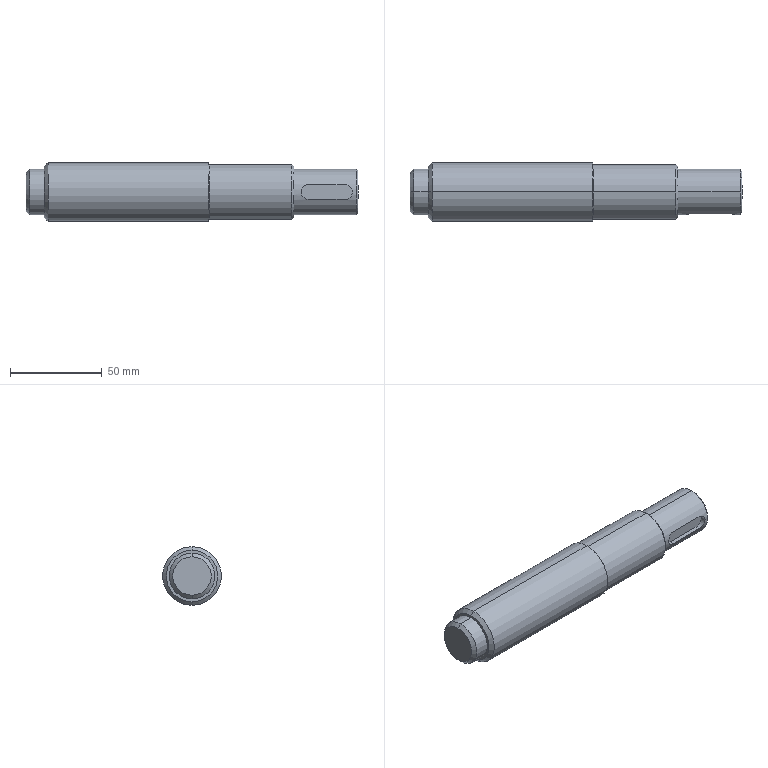Part | SolidWorks | features BaseBody 1 | 1 solid | 32 faces | box 181 x 32 x 32 mm | volume 124690 mm3 | cylinder 12 | cone 10 | plane 8 | spline 2 | commonest cylinder face diameters 25 x4 6.647 x2 8 x2 30 x2 32 x2
STEP:
#1=CARTESIAN_POINT('',(99.5,0.,15.5));
#2=VERTEX_POINT('',#1);
#3=CARTESIAN_POINT('',(99.5,0.,-15.5));
#4=VERTEX_POINT('',#3);
#5=CARTESIAN_POINT('',(99.5,0.,15.5));
#6=CARTESIAN_POINT('',(99.5,0.4739,15.5));
#7=CARTESIAN_POINT('',(99.5,1.182,15.468));
#8=CARTESIAN_POINT('',(99.5,2.003,15.373));
#9=CARTESIAN_POINT('',(99.5,2.412,15.312));
#10=CARTESIAN_POINT('',(99.5,2.616,15.278));
#11=CARTESIAN_POINT('',(99.5,2.704,15.262));
#12=CARTESIAN_POINT('',(99.5,2.762,15.252));
#13=CARTESIAN_POINT('',(99.5,2.79,15.247));
#14=CARTESIAN_POINT('',(99.5,3.315,15.15));
#15=CARTESIAN_POINT('',(99.5,4.046,14.978));
#16=CARTESIAN_POINT('',(99.5,4.881,14.715));
#17=CARTESIAN_POINT('',(99.5,5.295,14.569));
#18=CARTESIAN_POINT('',(99.5,5.501,14.491));
#19=CARTESIAN_POINT('',(99.5,5.588,14.458));
#20=CARTESIAN_POINT('',(99.5,5.647,14.435));
#21=CARTESIAN_POINT('',(99.5,5.675,14.424));
#22=CARTESIAN_POINT('',(99.5,6.192,14.219));
#23=CARTESIAN_POINT('',(99.5,6.905,13.895));
#24=CARTESIAN_POINT('',(99.5,7.704,13.455));
#25=CARTESIAN_POINT('',(99.5,8.095,13.219));
#26=CARTESIAN_POINT('',(99.5,8.262,13.115));
#27=CARTESIAN_POINT('',(99.5,8.372,13.045));
#28=CARTESIAN_POINT('',(99.5,8.426,13.01));
#29=CARTESIAN_POINT('',(99.5,9.377,12.388));
#30=CARTESIAN_POINT('',(99.5,10.204,11.717));
#31=CARTESIAN_POINT('',(99.5,11.338,10.582));
#32=CARTESIAN_POINT('',(99.5,11.874,9.989));
#33=CARTESIAN_POINT('',(99.5,12.442,9.25));
#34=CARTESIAN_POINT('',(99.5,12.712,8.87));
#35=CARTESIAN_POINT('',(99.5,12.825,8.704));
#36=CARTESIAN_POINT('',(99.5,12.9,8.593));
#37=CARTESIAN_POINT('',(99.5,12.938,8.537));
#38=CARTESIAN_POINT('',(99.5,13.26,8.043));
#39=CARTESIAN_POINT('',(99.5,13.655,7.368));
#40=CARTESIAN_POINT('',(99.5,14.054,6.547));
#41=CARTESIAN_POINT('',(99.5,14.238,6.129));
#42=CARTESIAN_POINT('',(99.5,14.326,5.918));
#43=CARTESIAN_POINT('',(99.5,14.363,5.827));
#44=CARTESIAN_POINT('',(99.5,14.388,5.766));
#45=CARTESIAN_POINT('',(99.5,14.4,5.735));
#46=CARTESIAN_POINT('',(99.5,14.597,5.238));
#47=CARTESIAN_POINT('',(99.5,14.839,4.527));
#48=CARTESIAN_POINT('',(99.5,15.061,3.68));
#49=CARTESIAN_POINT('',(99.5,15.156,3.252));
#50=CARTESIAN_POINT('',(99.5,15.2,3.036));
#51=CARTESIAN_POINT('',(99.5,15.218,2.944));
#52=CARTESIAN_POINT('',(99.5,15.23,2.882));
#53=CARTESIAN_POINT('',(99.5,15.236,2.85));
#54=CARTESIAN_POINT('',(99.5,15.414,1.888));
#55=CARTESIAN_POINT('',(99.5,15.5,0.9479));
#56=CARTESIAN_POINT('',(99.5,15.5,-0.4739));
#57=CARTESIAN_POINT('',(99.5,15.478,-0.9462));
#58=CARTESIAN_POINT('',(99.5,15.414,-1.651));
#59=CARTESIAN_POINT('',(99.5,15.373,-2.003));
#60=CARTESIAN_POINT('',(99.5,15.312,-2.412));
#61=CARTESIAN_POINT('',(99.5,15.278,-2.616));
#62=CARTESIAN_POINT('',(99.5,15.262,-2.704));
#63=CARTESIAN_POINT('',(99.5,15.252,-2.762));
#64=CARTESIAN_POINT('',(99.5,15.247,-2.79));
#65=CARTESIAN_POINT('',(99.5,15.15,-3.315));
#66=CARTESIAN_POINT('',(99.5,14.978,-4.046));
#67=CARTESIAN_POINT('',(99.5,14.715,-4.881));
#68=CARTESIAN_POINT('',(99.5,14.569,-5.295));
#69=CARTESIAN_POINT('',(99.5,14.491,-5.501));
#70=CARTESIAN_POINT('',(99.5,14.458,-5.588));
#71=CARTESIAN_POINT('',(99.5,14.435,-5.647));
#72=CARTESIAN_POINT('',(99.5,14.424,-5.675));
#73=CARTESIAN_POINT('',(99.5,14.219,-6.192));
#74=CARTESIAN_POINT('',(99.5,13.895,-6.905));
#75=CARTESIAN_POINT('',(99.5,13.455,-7.704));
#76=CARTESIAN_POINT('',(99.5,13.219,-8.095));
#77=CARTESIAN_POINT('',(99.5,13.115,-8.262));
#78=CARTESIAN_POINT('',(99.5,13.045,-8.372));
#79=CARTESIAN_POINT('',(99.5,13.01,-8.426));
#80=CARTESIAN_POINT('',(99.5,12.388,-9.377));
#81=CARTESIAN_POINT('',(99.5,11.717,-10.204));
#82=CARTESIAN_POINT('',(99.5,10.582,-11.338));
#83=CARTESIAN_POINT('',(99.5,9.989,-11.874));
#84=CARTESIAN_POINT('',(99.5,9.25,-12.442));
#85=CARTESIAN_POINT('',(99.5,8.87,-12.712));
#86=CARTESIAN_POINT('',(99.5,8.704,-12.825));
#87=CARTESIAN_POINT('',(99.5,8.593,-12.9));
#88=CARTESIAN_POINT('',(99.5,8.537,-12.938));
#89=CARTESIAN_POINT('',(99.5,8.043,-13.26));
#90=CARTESIAN_POINT('',(99.5,7.368,-13.655));
#91=CARTESIAN_POINT('',(99.5,6.547,-14.054));
#92=CARTESIAN_POINT('',(99.5,6.129,-14.238));
#93=CARTESIAN_POINT('',(99.5,5.918,-14.326));
#94=CARTESIAN_POINT('',(99.5,5.827,-14.363));
#95=CARTESIAN_POINT('',(99.5,5.766,-14.388));
#96=CARTESIAN_POINT('',(99.5,5.735,-14.4));
#97=CARTESIAN_POINT('',(99.5,5.238,-14.597));
#98=CARTESIAN_POINT('',(99.5,4.527,-14.839));
#99=CARTESIAN_POINT('',(99.5,3.68,-15.061));
#100=CARTESIAN_POINT('',(99.5,3.252,-15.156));
#101=CARTESIAN_POINT('',(99.5,3.036,-15.2));
#102=CARTESIAN_POINT('',(99.5,2.944,-15.218));
#103=CARTESIAN_POINT('',(99.5,2.882,-15.23));
#104=CARTESIAN_POINT('',(99.5,2.85,-15.236));
#105=CARTESIAN_POINT('',(99.5,1.889,-15.414));
#106=CARTESIAN_POINT('',(99.5,0.9477,-15.5));
#107=CARTESIAN_POINT('',(99.5,0.,-15.5));
#108=B_SPLINE_CURVE_WITH_KNOTS('',3,(#5,#6,#7,#8,#9,#10,#11,#12,#13,#14,#15,#16,#17,#18,#19,#20,#21,#22,#23,#24,#25,#26,#27,#28,#29,#30,#31,#32,#33,#34,#35,#36,#37,#38,#39,#40,#41,#42,#43,#44,#45,#46,#47,#48,#49,#50,#51,#52,#53,#54,#55,#56,#57,#58,#59,#60,#61,#62,#63,#64,#65,#66,#67,#68,#69,#70,#71,#72,#73,#74,#75,#76,#77,#78,#79,#80,#81,#82,#83,#84,#85,#86,#87,#88,#89,#90,#91,#92,#93,#94,#95,#96,#97,#98,#99,#100,#101,#102,#103,#104,#105,#106,#107),.UNSPECIFIED.,.F.,.F.,(4,1,1,1,1,2,2,1,1,1,1,2,2,1,1,1,2,2,2,1,1,1,2,2,1,1,1,1,2,2,1,1,1,1,2,2,2,2,1,1,1,2,2,1,1,1,1,2,2,1,1,1,2,2,2,1,1,1,2,2,1,1,1,1,2,2,1,1,1,1,2,2,4),(0.75,0.7656,0.7734,0.7773,0.7793,0.7803,0.7813,0.7969,0.8047,0.8086,0.8105,0.8115,0.8125,0.8281,0.8359,0.8398,0.8418,0.8438,0.875,0.8906,0.8984,0.9023,0.9043,0.9063,0.9219,0.9297,0.9336,0.9355,0.9365,0.9375,0.9531,0.9609,0.9648,0.9668,0.9678,0.9688,1.,1.016,1.023,1.027,1.029,1.03,1.031,1.047,1.055,1.059,1.061,1.062,1.063,1.078,1.086,1.09,1.092,1.094,1.125,1.141,1.148,1.152,1.154,1.156,1.172,1.18,1.184,1.186,1.187,1.188,1.203,1.211,1.215,1.217,1.218,1.219,1.25),.UNSPECIFIED.);
#109=EDGE_CURVE('',#2,#4,#108,.T.);
#110=ORIENTED_EDGE('',*,*,#109,.F.);
#111=CARTESIAN_POINT('',(100.,0.,15.));
#112=VERTEX_POINT('',#111);
#113=CARTESIAN_POINT('',(100.,0.,15.5));
#114=DIRECTION('',(0.,-1.,0.));
#115=DIRECTION('',(0.,0.,1.));
#116=AXIS2_PLACEMENT_3D('',#113,#114,#115);
#117=CIRCLE('',#116,0.5);
#118=EDGE_CURVE('',#2,#112,#117,.T.);
#119=ORIENTED_EDGE('',*,*,#118,.T.);
#120=CARTESIAN_POINT('',(100.,0.,-15.));
#121=VERTEX_POINT('',#120);
#122=CARTESIAN_POINT('',(100.,0.,0.));
#123=DIRECTION('',(1.,0.,0.));
#124=DIRECTION('',(0.,0.,-1.));
#125=AXIS2_PLACEMENT_3D('',#122,#123,#124);
#126=CIRCLE('',#125,15.);
#127=EDGE_CURVE('',#121,#112,#126,.T.);
#128=ORIENTED_EDGE('',*,*,#127,.F.);
#129=CARTESIAN_POINT('',(100.,0.,-15.5));
#130=DIRECTION('',(0.,1.,0.));
#131=DIRECTION('',(0.,0.,-1.));
#132=AXIS2_PLACEMENT_3D('',#129,#130,#131);
#133=CIRCLE('',#132,0.5);
#134=EDGE_CURVE('',#4,#121,#133,.T.);
#135=ORIENTED_EDGE('',*,*,#134,.F.);
#136=EDGE_LOOP('',(#110,#119,#128,#135));
#137=FACE_OUTER_BOUND('',#136,.T.);
#138=CARTESIAN_POINT('',(99.5,0.,-15.5));
#139=CARTESIAN_POINT('',(99.5,31.,-15.5));
#140=CARTESIAN_POINT('',(99.5,31.,15.5));
#141=CARTESIAN_POINT('',(99.5,0.,15.5));
#142=CARTESIAN_POINT('',(99.5,0.,-15.207));
#143=CARTESIAN_POINT('',(99.5,30.414,-15.207));
#144=CARTESIAN_POINT('',(99.5,30.414,15.207));
#145=CARTESIAN_POINT('',(99.5,0.,15.207));
#146=CARTESIAN_POINT('',(99.707,0.,-15.));
#147=CARTESIAN_POINT('',(99.707,30.,-15.));
#148=CARTESIAN_POINT('',(99.707,30.,15.));
#149=CARTESIAN_POINT('',(99.707,0.,15.));
#150=CARTESIAN_POINT('',(100.,0.,-15.));
#151=CARTESIAN_POINT('',(100.,30.,-15.));
#152=CARTESIAN_POINT('',(100.,30.,15.));
#153=CARTESIAN_POINT('',(100.,0.,15.));
#154=(BOUNDED_SURFACE()B_SPLINE_SURFACE(3,3,((#138,#139,#140,#141),(#142,#143,#144,#145),(#146,#147,#148,#149),(#150,#151,#152,#153)),.UNSPECIFIED.,.F.,.F.,.T.)B_SPLINE_SURFACE_WITH_KNOTS((4,4),(4,4),(0.,1.),(0.,1.),.UNSPECIFIED.)GEOMETRIC_REPRESENTATION_ITEM()RATIONAL_B_SPLINE_SURFACE(((1.,0.3333,0.3333,1.),(0.8047,0.2682,0.2682,0.8047),(0.8047,0.2682,0.2682,0.8047),(1.,0.3333,0.3333,1.)))REPRESENTATION_ITEM('')SURFACE());
#155=ADVANCED_FACE('',(#137),#154,.F.);
#156=CARTESIAN_POINT('',(12.,0.,-16.));
#157=VERTEX_POINT('',#156);
#158=CARTESIAN_POINT('',(12.,0.,16.));
#159=VERTEX_POINT('',#158);
#160=CARTESIAN_POINT('',(12.,0.,0.));
#161=DIRECTION('',(1.,0.,0.));
#162=DIRECTION('',(0.,0.,-1.));
#163=AXIS2_PLACEMENT_3D('',#160,#161,#162);
#164=CIRCLE('',#163,16.);
#165=EDGE_CURVE('',#157,#159,#164,.T.);
#166=ORIENTED_EDGE('',*,*,#165,.T.);
#167=CARTESIAN_POINT('',(99.5,0.,16.));
#168=VERTEX_POINT('',#167);
#169=CARTESIAN_POINT('',(54.75,0.,16.));
#170=DIRECTION('',(1.,0.,0.));
#171=VECTOR('',#170,1000.);
#172=LINE('',#169,#171);
#173=EDGE_CURVE('',#159,#168,#172,.T.);
#174=ORIENTED_EDGE('',*,*,#173,.T.);
#175=CARTESIAN_POINT('',(99.5,0.,-16.));
#176=VERTEX_POINT('',#175);
#177=CARTESIAN_POINT('',(99.5,0.,0.));
#178=DIRECTION('',(-1.,0.,0.));
#179=DIRECTION('',(0.,0.,-1.));
#180=AXIS2_PLACEMENT_3D('',#177,#178,#179);
#181=CIRCLE('',#180,16.);
#182=EDGE_CURVE('',#168,#176,#181,.T.);
#183=ORIENTED_EDGE('',*,*,#182,.T.);
#184=CARTESIAN_POINT('',(54.75,0.,-16.));
#185=DIRECTION('',(1.,0.,0.));
#186=VECTOR('',#185,1000.);
#187=LINE('',#184,#186);
#188=EDGE_CURVE('',#157,#176,#187,.T.);
#189=ORIENTED_EDGE('',*,*,#188,.F.);
#190=EDGE_LOOP('',(#166,#174,#183,#189));
#191=FACE_OUTER_BOUND('',#190,.T.);
#192=CARTESIAN_POINT('',(54.75,0.,0.));
#193=DIRECTION('',(1.,0.,0.));
#194=DIRECTION('',(0.,0.,-1.));
#195=AXIS2_PLACEMENT_3D('',#192,#193,#194);
#196=CYLINDRICAL_SURFACE('',#195,16.);
#197=ADVANCED_FACE('',(#191),#196,.T.);
#198=CARTESIAN_POINT('',(10.,0.,-14.));
#199=VERTEX_POINT('',#198);
#200=CARTESIAN_POINT('',(10.,0.,14.));
#201=VERTEX_POINT('',#200);
#202=CARTESIAN_POINT('',(10.,0.,0.));
#203=DIRECTION('',(1.,0.,0.));
#204=DIRECTION('',(0.,0.,-1.));
#205=AXIS2_PLACEMENT_3D('',#202,#203,#204);
#206=CIRCLE('',#205,14.);
#207=EDGE_CURVE('',#199,#201,#206,.T.);
#208=ORIENTED_EDGE('',*,*,#207,.T.);
#209=CARTESIAN_POINT('',(12.,0.,16.));
#210=DIRECTION('',(0.7071,0.,0.7071));
#211=VECTOR('',#210,1000.);
#212=LINE('',#209,#211);
#213=EDGE_CURVE('',#201,#159,#212,.T.);
#214=ORIENTED_EDGE('',*,*,#213,.T.);
#215=ORIENTED_EDGE('',*,*,#165,.F.);
#216=CARTESIAN_POINT('',(12.,0.,-16.));
#217=DIRECTION('',(0.7071,0.,-0.7071));
#218=VECTOR('',#217,1000.);
#219=LINE('',#216,#218);
#220=EDGE_CURVE('',#199,#157,#219,.T.);
#221=ORIENTED_EDGE('',*,*,#220,.F.);
#222=EDGE_LOOP('',(#208,#214,#215,#221));
#223=FACE_OUTER_BOUND('',#222,.T.);
#224=CARTESIAN_POINT('',(12.,0.,0.));
#225=DIRECTION('',(1.,0.,0.));
#226=DIRECTION('',(0.,0.,-1.));
#227=AXIS2_PLACEMENT_3D('',#224,#225,#226);
#228=CONICAL_SURFACE('',#227,16.,0.7854);
#229=ADVANCED_FACE('',(#223),#228,.T.);
#230=CARTESIAN_POINT('',(2.,0.,-12.5));
#231=VERTEX_POINT('',#230);
#232=CARTESIAN_POINT('',(2.,0.,12.5));
#233=VERTEX_POINT('',#232);
#234=CARTESIAN_POINT('',(2.,0.,0.));
#235=DIRECTION('',(1.,0.,0.));
#236=DIRECTION('',(0.,0.,-1.));
#237=AXIS2_PLACEMENT_3D('',#234,#235,#236);
#238=CIRCLE('',#237,12.5);
#239=EDGE_CURVE('',#231,#233,#238,.T.);
#240=ORIENTED_EDGE('',*,*,#239,.T.);
#241=CARTESIAN_POINT('',(10.,0.,12.5));
#242=VERTEX_POINT('',#241);
#243=CARTESIAN_POINT('',(5.,0.,12.5));
#244=DIRECTION('',(1.,0.,0.));
#245=VECTOR('',#244,1000.);
#246=LINE('',#243,#245);
#247=EDGE_CURVE('',#233,#242,#246,.T.);
#248=ORIENTED_EDGE('',*,*,#247,.T.);
#249=CARTESIAN_POINT('',(10.,0.,-12.5));
#250=VERTEX_POINT('',#249);
#251=CARTESIAN_POINT('',(10.,0.,0.));
#252=DIRECTION('',(1.,0.,0.));
#253=DIRECTION('',(0.,0.,-1.));
#254=AXIS2_PLACEMENT_3D('',#251,#252,#253);
#255=CIRCLE('',#254,12.5);
#256=EDGE_CURVE('',#250,#242,#255,.T.);
#257=ORIENTED_EDGE('',*,*,#256,.F.);
#258=CARTESIAN_POINT('',(5.,0.,-12.5));
#259=DIRECTION('',(1.,0.,0.));
#260=VECTOR('',#259,1000.);
#261=LINE('',#258,#260);
#262=EDGE_CURVE('',#231,#250,#261,.T.);
#263=ORIENTED_EDGE('',*,*,#262,.F.);
#264=EDGE_LOOP('',(#240,#248,#257,#263));
#265=FACE_OUTER_BOUND('',#264,.T.);
#266=CARTESIAN_POINT('',(5.,0.,0.));
#267=DIRECTION('',(1.,0.,0.));
#268=DIRECTION('',(0.,0.,-1.));
#269=AXIS2_PLACEMENT_3D('',#266,#267,#268);
#270=CYLINDRICAL_SURFACE('',#269,12.5);
#271=ADVANCED_FACE('',(#265),#270,.T.);
#272=ORIENTED_EDGE('',*,*,#127,.T.);
#273=CARTESIAN_POINT('',(145.,0.,15.));
#274=VERTEX_POINT('',#273);
#275=CARTESIAN_POINT('',(141.75,0.,15.));
#276=DIRECTION('',(1.,0.,0.));
#277=VECTOR('',#276,1000.);
#278=LINE('',#275,#277);
#279=EDGE_CURVE('',#112,#274,#278,.T.);
#280=ORIENTED_EDGE('',*,*,#279,.T.);
#281=CARTESIAN_POINT('',(145.,0.,-15.));
#282=VERTEX_POINT('',#281);
#283=CARTESIAN_POINT('',(145.,0.,0.));
#284=DIRECTION('',(-1.,0.,0.));
#285=DIRECTION('',(0.,0.,-1.));
#286=AXIS2_PLACEMENT_3D('',#283,#284,#285);
#287=CIRCLE('',#286,15.);
#288=EDGE_CURVE('',#274,#282,#287,.T.);
#289=ORIENTED_EDGE('',*,*,#288,.T.);
#290=CARTESIAN_POINT('',(141.75,0.,-15.));
#291=DIRECTION('',(1.,0.,0.));
#292=VECTOR('',#291,1000.);
#293=LINE('',#290,#292);
#294=EDGE_CURVE('',#121,#282,#293,.T.);
#295=ORIENTED_EDGE('',*,*,#294,.F.);
#296=EDGE_LOOP('',(#272,#280,#289,#295));
#297=FACE_OUTER_BOUND('',#296,.T.);
#298=CARTESIAN_POINT('',(141.75,0.,0.));
#299=DIRECTION('',(1.,0.,0.));
#300=DIRECTION('',(0.,0.,-1.));
#301=AXIS2_PLACEMENT_3D('',#298,#299,#300);
#302=CYLINDRICAL_SURFACE('',#301,15.);
#303=ADVANCED_FACE('',(#297),#302,.T.);
#304=CARTESIAN_POINT('',(0.,0.,-10.5));
#305=VERTEX_POINT('',#304);
#306=CARTESIAN_POINT('',(0.,0.,10.5));
#307=VERTEX_POINT('',#306);
#308=CARTESIAN_POINT('',(0.,0.,0.));
#309=DIRECTION('',(1.,0.,0.));
#310=DIRECTION('',(0.,0.,-1.));
#311=AXIS2_PLACEMENT_3D('',#308,#309,#310);
#312=CIRCLE('',#311,10.5);
#313=EDGE_CURVE('',#305,#307,#312,.T.);
#314=ORIENTED_EDGE('',*,*,#313,.T.);
#315=CARTESIAN_POINT('',(2.,0.,12.5));
#316=DIRECTION('',(0.7071,0.,0.7071));
#317=VECTOR('',#316,1000.);
#318=LINE('',#315,#317);
#319=EDGE_CURVE('',#307,#233,#318,.T.);
#320=ORIENTED_EDGE('',*,*,#319,.T.);
#321=ORIENTED_EDGE('',*,*,#239,.F.);
#322=CARTESIAN_POINT('',(2.,0.,-12.5));
#323=DIRECTION('',(0.7071,0.,-0.7071));
#324=VECTOR('',#323,1000.);
#325=LINE('',#322,#324);
#326=EDGE_CURVE('',#305,#231,#325,.T.);
#327=ORIENTED_EDGE('',*,*,#326,.F.);
#328=EDGE_LOOP('',(#314,#320,#321,#327));
#329=FACE_OUTER_BOUND('',#328,.T.);
#330=CARTESIAN_POINT('',(2.,0.,0.));
#331=DIRECTION('',(1.,0.,0.));
#332=DIRECTION('',(0.,0.,-1.));
#333=AXIS2_PLACEMENT_3D('',#330,#331,#332);
#334=CONICAL_SURFACE('',#333,12.5,0.7854);
#335=ADVANCED_FACE('',(#329),#334,.T.);
#336=CARTESIAN_POINT('',(146.,0.,14.));
#337=VERTEX_POINT('',#336);
#338=CARTESIAN_POINT('',(146.,0.,-14.));
#339=VERTEX_POINT('',#338);
#340=CARTESIAN_POINT('',(146.,0.,0.));
#341=DIRECTION('',(-1.,0.,0.));
#342=DIRECTION('',(0.,0.,1.));
#343=AXIS2_PLACEMENT_3D('',#340,#341,#342);
#344=CIRCLE('',#343,14.);
#345=EDGE_CURVE('',#337,#339,#344,.T.);
#346=ORIENTED_EDGE('',*,*,#345,.T.);
#347=CARTESIAN_POINT('',(145.,0.,-15.));
#348=DIRECTION('',(-0.7071,0.,-0.7071));
#349=VECTOR('',#348,1000.);
#350=LINE('',#347,#349);
#351=EDGE_CURVE('',#339,#282,#350,.T.);
#352=ORIENTED_EDGE('',*,*,#351,.T.);
#353=ORIENTED_EDGE('',*,*,#288,.F.);
#354=CARTESIAN_POINT('',(145.,0.,15.));
#355=DIRECTION('',(-0.7071,0.,0.7071));
#356=VECTOR('',#355,1000.);
#357=LINE('',#354,#356);
#358=EDGE_CURVE('',#337,#274,#357,.T.);
#359=ORIENTED_EDGE('',*,*,#358,.F.);
#360=EDGE_LOOP('',(#346,#352,#353,#359));
#361=FACE_OUTER_BOUND('',#360,.T.);
#362=CARTESIAN_POINT('',(145.,0.,0.));
#363=DIRECTION('',(-1.,0.,0.));
#364=DIRECTION('',(0.,0.,1.));
#365=AXIS2_PLACEMENT_3D('',#362,#363,#364);
#366=CONICAL_SURFACE('',#365,15.,0.7854);
#367=ADVANCED_FACE('',(#361),#366,.T.);
#368=CARTESIAN_POINT('',(146.,0.,12.5));
#369=VERTEX_POINT('',#368);
#370=CARTESIAN_POINT('',(146.,0.,-12.5));
#371=VERTEX_POINT('',#370);
#372=CARTESIAN_POINT('',(146.,0.,0.));
#373=DIRECTION('',(-1.,0.,0.));
#374=DIRECTION('',(0.,0.,-1.));
#375=AXIS2_PLACEMENT_3D('',#372,#373,#374);
#376=CIRCLE('',#375,12.5);
#377=EDGE_CURVE('',#369,#371,#376,.T.);
#378=ORIENTED_EDGE('',*,*,#377,.F.);
#379=CARTESIAN_POINT('',(180.,0.,12.5));
#380=VERTEX_POINT('',#379);
#381=CARTESIAN_POINT('',(163.5,0.,12.5));
#382=DIRECTION('',(1.,0.,0.));
#383=VECTOR('',#382,1000.);
#384=LINE('',#381,#383);
#385=EDGE_CURVE('',#369,#380,#384,.T.);
#386=ORIENTED_EDGE('',*,*,#385,.T.);
#387=CARTESIAN_POINT('',(180.,0.,-12.5));
#388=VERTEX_POINT('',#387);
#389=CARTESIAN_POINT('',(180.,0.,0.));
#390=DIRECTION('',(-1.,0.,0.));
#391=DIRECTION('',(0.,0.,-1.));
#392=AXIS2_PLACEMENT_3D('',#389,#390,#391);
#393=CIRCLE('',#392,12.5);
#394=EDGE_CURVE('',#380,#388,#393,.T.);
#395=ORIENTED_EDGE('',*,*,#394,.T.);
#396=CARTESIAN_POINT('',(163.5,0.,-12.5));
#397=DIRECTION('',(1.,0.,0.));
#398=VECTOR('',#397,1000.);
#399=LINE('',#396,#398);
#400=EDGE_CURVE('',#371,#388,#399,.T.);
#401=ORIENTED_EDGE('',*,*,#400,.F.);
#402=EDGE_LOOP('',(#378,#386,#395,#401));
#403=FACE_OUTER_BOUND('',#402,.T.);
#404=CARTESIAN_POINT('',(163.5,0.,0.));
#405=DIRECTION('',(1.,0.,0.));
#406=DIRECTION('',(0.,0.,-1.));
#407=AXIS2_PLACEMENT_3D('',#404,#405,#406);
#408=CYLINDRICAL_SURFACE('',#407,12.5);
#409=ADVANCED_FACE('',(#403),#408,.T.);
#410=CARTESIAN_POINT('',(181.,0.,11.5));
#411=VERTEX_POINT('',#410);
#412=CARTESIAN_POINT('',(181.,0.,-11.5));
#413=VERTEX_POINT('',#412);
#414=CARTESIAN_POINT('',(181.,0.,0.));
#415=DIRECTION('',(-1.,0.,0.));
#416=DIRECTION('',(0.,0.,1.));
#417=AXIS2_PLACEMENT_3D('',#414,#415,#416);
#418=CIRCLE('',#417,11.5);
#419=EDGE_CURVE('',#411,#413,#418,.T.);
#420=ORIENTED_EDGE('',*,*,#419,.T.);
#421=CARTESIAN_POINT('',(180.,0.,-12.5));
#422=DIRECTION('',(-0.7071,0.,-0.7071));
#423=VECTOR('',#422,1000.);
#424=LINE('',#421,#423);
#425=EDGE_CURVE('',#413,#388,#424,.T.);
#426=ORIENTED_EDGE('',*,*,#425,.T.);
#427=ORIENTED_EDGE('',*,*,#394,.F.);
#428=CARTESIAN_POINT('',(180.,0.,12.5));
#429=DIRECTION('',(-0.7071,0.,0.7071));
#430=VECTOR('',#429,1000.);
#431=LINE('',#428,#430);
#432=EDGE_CURVE('',#411,#380,#431,.T.);
#433=ORIENTED_EDGE('',*,*,#432,.F.);
#434=EDGE_LOOP('',(#420,#426,#427,#433));
#435=FACE_OUTER_BOUND('',#434,.T.);
#436=CARTESIAN_POINT('',(180.,0.,0.));
#437=DIRECTION('',(-1.,0.,0.));
#438=DIRECTION('',(0.,0.,1.));
#439=AXIS2_PLACEMENT_3D('',#436,#437,#438);
#440=CONICAL_SURFACE('',#439,12.5,0.7854);
#441=ADVANCED_FACE('',(#435),#440,.T.);
#442=CARTESIAN_POINT('',(146.,0.,3.323));
#443=VERTEX_POINT('',#442);
#444=CARTESIAN_POINT('',(146.,0.,-3.323));
#445=VERTEX_POINT('',#444);
#446=CARTESIAN_POINT('',(146.,0.,0.));
#447=DIRECTION('',(1.,0.,0.));
#448=DIRECTION('',(0.,0.,-1.));
#449=AXIS2_PLACEMENT_3D('',#446,#447,#448);
#450=CIRCLE('',#449,3.324);
#451=EDGE_CURVE('',#443,#445,#450,.T.);
#452=ORIENTED_EDGE('',*,*,#451,.F.);
#453=CARTESIAN_POINT('',(181.,0.,3.324));
#454=VERTEX_POINT('',#453);
#455=CARTESIAN_POINT('',(163.5,0.,3.324));
#456=DIRECTION('',(1.,0.,0.));
#457=VECTOR('',#456,1000.);
#458=LINE('',#455,#457);
#459=EDGE_CURVE('',#443,#454,#458,.T.);
#460=ORIENTED_EDGE('',*,*,#459,.T.);
#461=CARTESIAN_POINT('',(181.,0.,-3.324));
#462=VERTEX_POINT('',#461);
#463=CARTESIAN_POINT('',(181.,0.,0.));
#464=DIRECTION('',(-1.,0.,0.));
#465=DIRECTION('',(0.,0.,-1.));
#466=AXIS2_PLACEMENT_3D('',#463,#464,#465);
#467=CIRCLE('',#466,3.324);
#468=EDGE_CURVE('',#462,#454,#467,.T.);
#469=ORIENTED_EDGE('',*,*,#468,.F.);
#470=CARTESIAN_POINT('',(163.5,0.,-3.324));
#471=DIRECTION('',(1.,0.,0.));
#472=VECTOR('',#471,1000.);
#473=LINE('',#470,#472);
#474=EDGE_CURVE('',#445,#462,#473,.T.);
#475=ORIENTED_EDGE('',*,*,#474,.F.);
#476=EDGE_LOOP('',(#452,#460,#469,#475));
#477=FACE_OUTER_BOUND('',#476,.T.);
#478=CARTESIAN_POINT('',(163.5,0.,0.));
#479=DIRECTION('',(1.,0.,0.));
#480=DIRECTION('',(0.,0.,-1.));
#481=AXIS2_PLACEMENT_3D('',#478,#479,#480);
#482=CYLINDRICAL_SURFACE('',#481,3.324);
#483=ADVANCED_FACE('',(#477),#482,.F.);
#484=CARTESIAN_POINT('',(144.003,0.,0.));
#485=VERTEX_POINT('',#484);
#486=CARTESIAN_POINT('',(146.,0.,-3.323));
#487=DIRECTION('',(0.515,0.,-0.8572));
#488=VECTOR('',#487,1000.);
#489=LINE('',#486,#488);
#490=EDGE_CURVE('',#485,#445,#489,.T.);
#491=ORIENTED_EDGE('',*,*,#490,.F.);
#492=CARTESIAN_POINT('',(146.,0.,3.323));
#493=DIRECTION('',(0.515,0.,0.8572));
#494=VECTOR('',#493,1000.);
#495=LINE('',#492,#494);
#496=EDGE_CURVE('',#485,#443,#495,.T.);
#497=ORIENTED_EDGE('',*,*,#496,.T.);
#498=ORIENTED_EDGE('',*,*,#451,.T.);
#499=EDGE_LOOP('',(#491,#497,#498));
#500=FACE_OUTER_BOUND('',#499,.T.);
#501=CARTESIAN_POINT('',(146.,0.,0.));
#502=DIRECTION('',(1.,0.,0.));
#503=DIRECTION('',(0.,0.,-1.));
#504=AXIS2_PLACEMENT_3D('',#501,#502,#503);
#505=CONICAL_SURFACE('',#504,3.323,1.03);
#506=ADVANCED_FACE('',(#500),#505,.F.);
#507=ORIENTED_EDGE('',*,*,#173,.F.);
#508=CARTESIAN_POINT('',(12.,0.,0.));
#509=DIRECTION('',(1.,0.,0.));
#510=DIRECTION('',(0.,0.,-1.));
#511=AXIS2_PLACEMENT_3D('',#508,#509,#510);
#512=CIRCLE('',#511,16.);
#513=EDGE_CURVE('',#159,#157,#512,.T.);
#514=ORIENTED_EDGE('',*,*,#513,.T.);
#515=ORIENTED_EDGE('',*,*,#188,.T.);
#516=CARTESIAN_POINT('',(99.5,0.,0.));
#517=DIRECTION('',(-1.,0.,0.));
#518=DIRECTION('',(0.,0.,-1.));
#519=AXIS2_PLACEMENT_3D('',#516,#517,#518);
#520=CIRCLE('',#519,16.);
#521=EDGE_CURVE('',#176,#168,#520,.T.);
#522=ORIENTED_EDGE('',*,*,#521,.T.);
#523=EDGE_LOOP('',(#507,#514,#515,#522));
#524=FACE_OUTER_BOUND('',#523,.T.);
#525=CARTESIAN_POINT('',(54.75,0.,0.));
#526=DIRECTION('',(1.,0.,0.));
#527=DIRECTION('',(0.,0.,-1.));
#528=AXIS2_PLACEMENT_3D('',#525,#526,#527);
#529=CYLINDRICAL_SURFACE('',#528,16.);
#530=ADVANCED_FACE('',(#524),#529,.T.);
#531=ORIENTED_EDGE('',*,*,#213,.F.);
#532=CARTESIAN_POINT('',(10.,0.,0.));
#533=DIRECTION('',(1.,0.,0.));
#534=DIRECTION('',(0.,0.,-1.));
#535=AXIS2_PLACEMENT_3D('',#532,#533,#534);
#536=CIRCLE('',#535,14.);
#537=EDGE_CURVE('',#201,#199,#536,.T.);
#538=ORIENTED_EDGE('',*,*,#537,.T.);
#539=ORIENTED_EDGE('',*,*,#220,.T.);
#540=ORIENTED_EDGE('',*,*,#513,.F.);
#541=EDGE_LOOP('',(#531,#538,#539,#540));
#542=FACE_OUTER_BOUND('',#541,.T.);
#543=CARTESIAN_POINT('',(12.,0.,0.));
#544=DIRECTION('',(1.,0.,0.));
#545=DIRECTION('',(0.,0.,-1.));
#546=AXIS2_PLACEMENT_3D('',#543,#544,#545);
#547=CONICAL_SURFACE('',#546,16.,0.7854);
#548=ADVANCED_FACE('',(#542),#547,.T.);
#549=CARTESIAN_POINT('',(99.5,0.,-15.5));
#550=CARTESIAN_POINT('',(99.5,-0.4739,-15.5));
#551=CARTESIAN_POINT('',(99.5,-1.182,-15.468));
#552=CARTESIAN_POINT('',(99.5,-2.003,-15.373));
#553=CARTESIAN_POINT('',(99.5,-2.412,-15.312));
#554=CARTESIAN_POINT('',(99.5,-2.616,-15.278));
#555=CARTESIAN_POINT('',(99.5,-2.704,-15.262));
#556=CARTESIAN_POINT('',(99.5,-2.762,-15.252));
#557=CARTESIAN_POINT('',(99.5,-2.79,-15.247));
#558=CARTESIAN_POINT('',(99.5,-3.315,-15.15));
#559=CARTESIAN_POINT('',(99.5,-4.046,-14.978));
#560=CARTESIAN_POINT('',(99.5,-4.881,-14.715));
#561=CARTESIAN_POINT('',(99.5,-5.295,-14.569));
#562=CARTESIAN_POINT('',(99.5,-5.501,-14.491));
#563=CARTESIAN_POINT('',(99.5,-5.588,-14.458));
#564=CARTESIAN_POINT('',(99.5,-5.647,-14.435));
#565=CARTESIAN_POINT('',(99.5,-5.675,-14.424));
#566=CARTESIAN_POINT('',(99.5,-6.192,-14.219));
#567=CARTESIAN_POINT('',(99.5,-6.905,-13.895));
#568=CARTESIAN_POINT('',(99.5,-7.704,-13.455));
#569=CARTESIAN_POINT('',(99.5,-8.095,-13.219));
#570=CARTESIAN_POINT('',(99.5,-8.262,-13.115));
#571=CARTESIAN_POINT('',(99.5,-8.372,-13.045));
#572=CARTESIAN_POINT('',(99.5,-8.426,-13.01));
#573=CARTESIAN_POINT('',(99.5,-9.377,-12.388));
#574=CARTESIAN_POINT('',(99.5,-10.204,-11.717));
#575=CARTESIAN_POINT('',(99.5,-11.338,-10.582));
#576=CARTESIAN_POINT('',(99.5,-11.874,-9.989));
#577=CARTESIAN_POINT('',(99.5,-12.442,-9.25));
#578=CARTESIAN_POINT('',(99.5,-12.712,-8.87));
#579=CARTESIAN_POINT('',(99.5,-12.825,-8.704));
#580=CARTESIAN_POINT('',(99.5,-12.9,-8.593));
#581=CARTESIAN_POINT('',(99.5,-12.938,-8.537));
#582=CARTESIAN_POINT('',(99.5,-13.26,-8.043));
#583=CARTESIAN_POINT('',(99.5,-13.655,-7.368));
#584=CARTESIAN_POINT('',(99.5,-14.054,-6.547));
#585=CARTESIAN_POINT('',(99.5,-14.238,-6.129));
#586=CARTESIAN_POINT('',(99.5,-14.326,-5.918));
#587=CARTESIAN_POINT('',(99.5,-14.363,-5.827));
#588=CARTESIAN_POINT('',(99.5,-14.388,-5.766));
#589=CARTESIAN_POINT('',(99.5,-14.4,-5.735));
#590=CARTESIAN_POINT('',(99.5,-14.597,-5.238));
#591=CARTESIAN_POINT('',(99.5,-14.839,-4.527));
#592=CARTESIAN_POINT('',(99.5,-15.061,-3.68));
#593=CARTESIAN_POINT('',(99.5,-15.156,-3.252));
#594=CARTESIAN_POINT('',(99.5,-15.2,-3.036));
#595=CARTESIAN_POINT('',(99.5,-15.218,-2.944));
#596=CARTESIAN_POINT('',(99.5,-15.23,-2.882));
#597=CARTESIAN_POINT('',(99.5,-15.236,-2.85));
#598=CARTESIAN_POINT('',(99.5,-15.414,-1.889));
#599=CARTESIAN_POINT('',(99.5,-15.5,-0.9477));
#600=CARTESIAN_POINT('',(99.5,-15.5,0.4739));
#601=CARTESIAN_POINT('',(99.5,-15.468,1.182));
#602=CARTESIAN_POINT('',(99.5,-15.373,2.003));
#603=CARTESIAN_POINT('',(99.5,-15.312,2.412));
#604=CARTESIAN_POINT('',(99.5,-15.278,2.616));
#605=CARTESIAN_POINT('',(99.5,-15.262,2.704));
#606=CARTESIAN_POINT('',(99.5,-15.252,2.762));
#607=CARTESIAN_POINT('',(99.5,-15.247,2.79));
#608=CARTESIAN_POINT('',(99.5,-15.15,3.315));
#609=CARTESIAN_POINT('',(99.5,-14.978,4.046));
#610=CARTESIAN_POINT('',(99.5,-14.715,4.881));
#611=CARTESIAN_POINT('',(99.5,-14.569,5.295));
#612=CARTESIAN_POINT('',(99.5,-14.491,5.501));
#613=CARTESIAN_POINT('',(99.5,-14.458,5.588));
#614=CARTESIAN_POINT('',(99.5,-14.435,5.647));
#615=CARTESIAN_POINT('',(99.5,-14.424,5.675));
#616=CARTESIAN_POINT('',(99.5,-14.219,6.192));
#617=CARTESIAN_POINT('',(99.5,-13.895,6.905));
#618=CARTESIAN_POINT('',(99.5,-13.455,7.704));
#619=CARTESIAN_POINT('',(99.5,-13.219,8.095));
#620=CARTESIAN_POINT('',(99.5,-13.115,8.262));
#621=CARTESIAN_POINT('',(99.5,-13.045,8.372));
#622=CARTESIAN_POINT('',(99.5,-13.01,8.426));
#623=CARTESIAN_POINT('',(99.5,-12.388,9.377));
#624=CARTESIAN_POINT('',(99.5,-11.717,10.204));
#625=CARTESIAN_POINT('',(99.5,-10.582,11.338));
#626=CARTESIAN_POINT('',(99.5,-9.989,11.874));
#627=CARTESIAN_POINT('',(99.5,-9.25,12.442));
#628=CARTESIAN_POINT('',(99.5,-8.87,12.712));
#629=CARTESIAN_POINT('',(99.5,-8.704,12.825));
#630=CARTESIAN_POINT('',(99.5,-8.593,12.9));
#631=CARTESIAN_POINT('',(99.5,-8.537,12.938));
#632=CARTESIAN_POINT('',(99.5,-8.043,13.26));
#633=CARTESIAN_POINT('',(99.5,-7.368,13.655));
#634=CARTESIAN_POINT('',(99.5,-6.547,14.054));
#635=CARTESIAN_POINT('',(99.5,-6.129,14.238));
#636=CARTESIAN_POINT('',(99.5,-5.918,14.326));
#637=CARTESIAN_POINT('',(99.5,-5.827,14.363));
#638=CARTESIAN_POINT('',(99.5,-5.766,14.388));
#639=CARTESIAN_POINT('',(99.5,-5.735,14.4));
#640=CARTESIAN_POINT('',(99.5,-5.238,14.597));
#641=CARTESIAN_POINT('',(99.5,-4.527,14.839));
#642=CARTESIAN_POINT('',(99.5,-3.68,15.061));
#643=CARTESIAN_POINT('',(99.5,-3.252,15.156));
#644=CARTESIAN_POINT('',(99.5,-3.036,15.2));
#645=CARTESIAN_POINT('',(99.5,-2.944,15.218));
#646=CARTESIAN_POINT('',(99.5,-2.882,15.23));
#647=CARTESIAN_POINT('',(99.5,-2.85,15.236));
#648=CARTESIAN_POINT('',(99.5,-1.889,15.414));
#649=CARTESIAN_POINT('',(99.5,-0.9477,15.5));
#650=CARTESIAN_POINT('',(99.5,0.,15.5));
#651=B_SPLINE_CURVE_WITH_KNOTS('',3,(#549,#550,#551,#552,#553,#554,#555,#556,#557,#558,#559,#560,#561,#562,#563,#564,#565,#566,#567,#568,#569,#570,#571,#572,#573,#574,#575,#576,#577,#578,#579,#580,#581,#582,#583,#584,#585,#586,#587,#588,#589,#590,#591,#592,#593,#594,#595,#596,#597,#598,#599,#600,#601,#602,#603,#604,#605,#606,#607,#608,#609,#610,#611,#612,#613,#614,#615,#616,#617,#618,#619,#620,#621,#622,#623,#624,#625,#626,#627,#628,#629,#630,#631,#632,#633,#634,#635,#636,#637,#638,#639,#640,#641,#642,#643,#644,#645,#646,#647,#648,#649,#650),.UNSPECIFIED.,.F.,.F.,(4,1,1,1,1,2,2,1,1,1,1,2,2,1,1,1,2,2,2,1,1,1,2,2,1,1,1,1,2,2,1,1,1,1,2,2,2,1,1,1,1,2,2,1,1,1,1,2,2,1,1,1,2,2,2,1,1,1,2,2,1,1,1,1,2,2,1,1,1,1,2,2,4),(0.25,0.2656,0.2734,0.2773,0.2793,0.2803,0.2813,0.2969,0.3047,0.3086,0.3105,0.3115,0.3125,0.3281,0.3359,0.3398,0.3418,0.3438,0.375,0.3906,0.3984,0.4023,0.4043,0.4063,0.4219,0.4297,0.4336,0.4355,0.4365,0.4375,0.4531,0.4609,0.4648,0.4668,0.4678,0.4688,0.5,0.5156,0.5234,0.5273,0.5293,0.5303,0.5313,0.5469,0.5547,0.5586,0.5605,0.5615,0.5625,0.5781,0.5859,0.5898,0.5918,0.5938,0.625,0.6406,0.6484,0.6523,0.6543,0.6563,0.6719,0.6797,0.6836,0.6855,0.6865,0.6875,0.7031,0.7109,0.7148,0.7168,0.7178,0.7188,0.75),.UNSPECIFIED.);
#652=EDGE_CURVE('',#4,#2,#651,.T.);
#653=ORIENTED_EDGE('',*,*,#652,.T.);
#654=ORIENTED_EDGE('',*,*,#109,.T.);
#655=EDGE_LOOP('',(#653,#654));
#656=FACE_BOUND('',#655,.T.);
#657=ORIENTED_EDGE('',*,*,#521,.F.);
#658=ORIENTED_EDGE('',*,*,#182,.F.);
#659=EDGE_LOOP('',(#657,#658));
#660=FACE_OUTER_BOUND('',#659,.T.);
#661=CARTESIAN_POINT('',(99.5,15.5,0.));
#662=DIRECTION('',(1.,0.,0.));
#663=DIRECTION('',(0.,0.,-1.));
#664=AXIS2_PLACEMENT_3D('',#661,#662,#663);
#665=PLANE('',#664);
#666=ADVANCED_FACE('',(#656,#660),#665,.T.);
#667=ORIENTED_EDGE('',*,*,#256,.T.);
#668=CARTESIAN_POINT('',(10.,0.,0.));
#669=DIRECTION('',(1.,0.,0.));
#670=DIRECTION('',(0.,0.,-1.));
#671=AXIS2_PLACEMENT_3D('',#668,#669,#670);
#672=CIRCLE('',#671,12.5);
#673=EDGE_CURVE('',#242,#250,#672,.T.);
#674=ORIENTED_EDGE('',*,*,#673,.T.);
#675=EDGE_LOOP('',(#667,#674));
#676=FACE_BOUND('',#675,.T.);
#677=ORIENTED_EDGE('',*,*,#207,.F.);
#678=ORIENTED_EDGE('',*,*,#537,.F.);
#679=EDGE_LOOP('',(#677,#678));
#680=FACE_OUTER_BOUND('',#679,.T.);
#681=CARTESIAN_POINT('',(10.,16.,0.));
#682=DIRECTION('',(-1.,0.,0.));
#683=DIRECTION('',(0.,0.,1.));
#684=AXIS2_PLACEMENT_3D('',#681,#682,#683);
#685=PLANE('',#684);
#686=ADVANCED_FACE('',(#676,#680),#685,.T.);
#687=ORIENTED_EDGE('',*,*,#118,.F.);
#688=ORIENTED_EDGE('',*,*,#652,.F.);
#689=ORIENTED_EDGE('',*,*,#134,.T.);
#690=CARTESIAN_POINT('',(100.,0.,0.));
#691=DIRECTION('',(1.,0.,0.));
#692=DIRECTION('',(0.,0.,-1.));
#693=AXIS2_PLACEMENT_3D('',#690,#691,#692);
#694=CIRCLE('',#693,15.);
#695=EDGE_CURVE('',#112,#121,#694,.T.);
#696=ORIENTED_EDGE('',*,*,#695,.F.);
#697=EDGE_LOOP('',(#687,#688,#689,#696));
#698=FACE_OUTER_BOUND('',#697,.T.);
#699=CARTESIAN_POINT('',(99.5,0.,15.5));
#700=CARTESIAN_POINT('',(99.5,-31.,15.5));
#701=CARTESIAN_POINT('',(99.5,-31.,-15.5));
#702=CARTESIAN_POINT('',(99.5,0.,-15.5));
#703=CARTESIAN_POINT('',(99.5,0.,15.207));
#704=CARTESIAN_POINT('',(99.5,-30.414,15.207));
#705=CARTESIAN_POINT('',(99.5,-30.414,-15.207));
#706=CARTESIAN_POINT('',(99.5,0.,-15.207));
#707=CARTESIAN_POINT('',(99.707,0.,15.));
#708=CARTESIAN_POINT('',(99.707,-30.,15.));
#709=CARTESIAN_POINT('',(99.707,-30.,-15.));
#710=CARTESIAN_POINT('',(99.707,0.,-15.));
#711=CARTESIAN_POINT('',(100.,0.,15.));
#712=CARTESIAN_POINT('',(100.,-30.,15.));
#713=CARTESIAN_POINT('',(100.,-30.,-15.));
#714=CARTESIAN_POINT('',(100.,0.,-15.));
#715=(BOUNDED_SURFACE()B_SPLINE_SURFACE(3,3,((#699,#700,#701,#702),(#703,#704,#705,#706),(#707,#708,#709,#710),(#711,#712,#713,#714)),.UNSPECIFIED.,.F.,.F.,.F.)B_SPLINE_SURFACE_WITH_KNOTS((4,4),(4,4),(0.,1.),(0.,1.),.UNSPECIFIED.)GEOMETRIC_REPRESENTATION_ITEM()RATIONAL_B_SPLINE_SURFACE(((1.,0.3333,0.3333,1.),(0.8047,0.2682,0.2682,0.8047),(0.8047,0.2682,0.2682,0.8047),(1.,0.3333,0.3333,1.)))REPRESENTATION_ITEM('')SURFACE());
#716=ADVANCED_FACE('',(#698),#715,.F.);
#717=ORIENTED_EDGE('',*,*,#247,.F.);
#718=CARTESIAN_POINT('',(2.,0.,0.));
#719=DIRECTION('',(1.,0.,0.));
#720=DIRECTION('',(0.,0.,-1.));
#721=AXIS2_PLACEMENT_3D('',#718,#719,#720);
#722=CIRCLE('',#721,12.5);
#723=EDGE_CURVE('',#233,#231,#722,.T.);
#724=ORIENTED_EDGE('',*,*,#723,.T.);
#725=ORIENTED_EDGE('',*,*,#262,.T.);
#726=ORIENTED_EDGE('',*,*,#673,.F.);
#727=EDGE_LOOP('',(#717,#724,#725,#726));
#728=FACE_OUTER_BOUND('',#727,.T.);
#729=CARTESIAN_POINT('',(5.,0.,0.));
#730=DIRECTION('',(1.,0.,0.));
#731=DIRECTION('',(0.,0.,-1.));
#732=AXIS2_PLACEMENT_3D('',#729,#730,#731);
#733=CYLINDRICAL_SURFACE('',#732,12.5);
#734=ADVANCED_FACE('',(#728),#733,.T.);
#735=ORIENTED_EDGE('',*,*,#279,.F.);
#736=ORIENTED_EDGE('',*,*,#695,.T.);
#737=ORIENTED_EDGE('',*,*,#294,.T.);
#738=CARTESIAN_POINT('',(145.,0.,0.));
#739=DIRECTION('',(-1.,0.,0.));
#740=DIRECTION('',(0.,0.,-1.));
#741=AXIS2_PLACEMENT_3D('',#738,#739,#740);
#742=CIRCLE('',#741,15.);
#743=EDGE_CURVE('',#282,#274,#742,.T.);
#744=ORIENTED_EDGE('',*,*,#743,.T.);
#745=EDGE_LOOP('',(#735,#736,#737,#744));
#746=FACE_OUTER_BOUND('',#745,.T.);
#747=CARTESIAN_POINT('',(141.75,0.,0.));
#748=DIRECTION('',(1.,0.,0.));
#749=DIRECTION('',(0.,0.,-1.));
#750=AXIS2_PLACEMENT_3D('',#747,#748,#749);
#751=CYLINDRICAL_SURFACE('',#750,15.);
#752=ADVANCED_FACE('',(#746),#751,.T.);
#753=ORIENTED_EDGE('',*,*,#319,.F.);
#754=CARTESIAN_POINT('',(0.,0.,0.));
#755=DIRECTION('',(1.,0.,0.));
#756=DIRECTION('',(0.,0.,-1.));
#757=AXIS2_PLACEMENT_3D('',#754,#755,#756);
#758=CIRCLE('',#757,10.5);
#759=EDGE_CURVE('',#307,#305,#758,.T.);
#760=ORIENTED_EDGE('',*,*,#759,.T.);
#761=ORIENTED_EDGE('',*,*,#326,.T.);
#762=ORIENTED_EDGE('',*,*,#723,.F.);
#763=EDGE_LOOP('',(#753,#760,#761,#762));
#764=FACE_OUTER_BOUND('',#763,.T.);
#765=CARTESIAN_POINT('',(2.,0.,0.));
#766=DIRECTION('',(1.,0.,0.));
#767=DIRECTION('',(0.,0.,-1.));
#768=AXIS2_PLACEMENT_3D('',#765,#766,#767);
#769=CONICAL_SURFACE('',#768,12.5,0.7854);
#770=ADVANCED_FACE('',(#764),#769,.T.);
#771=ORIENTED_EDGE('',*,*,#351,.F.);
#772=CARTESIAN_POINT('',(146.,0.,0.));
#773=DIRECTION('',(-1.,0.,0.));
#774=DIRECTION('',(0.,0.,1.));
#775=AXIS2_PLACEMENT_3D('',#772,#773,#774);
#776=CIRCLE('',#775,14.);
#777=EDGE_CURVE('',#339,#337,#776,.T.);
#778=ORIENTED_EDGE('',*,*,#777,.T.);
#779=ORIENTED_EDGE('',*,*,#358,.T.);
#780=ORIENTED_EDGE('',*,*,#743,.F.);
#781=EDGE_LOOP('',(#771,#778,#779,#780));
#782=FACE_OUTER_BOUND('',#781,.T.);
#783=CARTESIAN_POINT('',(145.,0.,0.));
#784=DIRECTION('',(-1.,0.,0.));
#785=DIRECTION('',(0.,0.,1.));
#786=AXIS2_PLACEMENT_3D('',#783,#784,#785);
#787=CONICAL_SURFACE('',#786,15.,0.7854);
#788=ADVANCED_FACE('',(#782),#787,.T.);
#789=ORIENTED_EDGE('',*,*,#313,.F.);
#790=ORIENTED_EDGE('',*,*,#759,.F.);
#791=EDGE_LOOP('',(#789,#790));
#792=FACE_OUTER_BOUND('',#791,.T.);
#793=CARTESIAN_POINT('',(0.,12.5,0.));
#794=DIRECTION('',(-1.,0.,0.));
#795=DIRECTION('',(0.,0.,1.));
#796=AXIS2_PLACEMENT_3D('',#793,#794,#795);
#797=PLANE('',#796);
#798=ADVANCED_FACE('',(#792),#797,.T.);
#799=CARTESIAN_POINT('',(146.,0.,0.));
#800=DIRECTION('',(-1.,0.,0.));
#801=DIRECTION('',(0.,0.,-1.));
#802=AXIS2_PLACEMENT_3D('',#799,#800,#801);
#803=CIRCLE('',#802,12.5);
#804=EDGE_CURVE('',#371,#369,#803,.T.);
#805=ORIENTED_EDGE('',*,*,#804,.T.);
#806=ORIENTED_EDGE('',*,*,#377,.T.);
#807=EDGE_LOOP('',(#805,#806));
#808=FACE_BOUND('',#807,.T.);
#809=ORIENTED_EDGE('',*,*,#345,.F.);
#810=ORIENTED_EDGE('',*,*,#777,.F.);
#811=EDGE_LOOP('',(#809,#810));
#812=FACE_OUTER_BOUND('',#811,.T.);
#813=CARTESIAN_POINT('',(146.,12.5,0.));
#814=DIRECTION('',(1.,0.,0.));
#815=DIRECTION('',(0.,0.,-1.));
#816=AXIS2_PLACEMENT_3D('',#813,#814,#815);
#817=PLANE('',#816);
#818=ADVANCED_FACE('',(#808,#812),#817,.T.);
#819=ORIENTED_EDGE('',*,*,#385,.F.);
#820=ORIENTED_EDGE('',*,*,#804,.F.);
#821=ORIENTED_EDGE('',*,*,#400,.T.);
#822=CARTESIAN_POINT('',(180.,0.,0.));
#823=DIRECTION('',(-1.,0.,0.));
#824=DIRECTION('',(0.,0.,-1.));
#825=AXIS2_PLACEMENT_3D('',#822,#823,#824);
#826=CIRCLE('',#825,12.5);
#827=EDGE_CURVE('',#388,#380,#826,.T.);
#828=ORIENTED_EDGE('',*,*,#827,.T.);
#829=EDGE_LOOP('',(#819,#820,#821,#828));
#830=FACE_OUTER_BOUND('',#829,.T.);
#831=CARTESIAN_POINT('',(174.,-11.843,-4.));
#832=VERTEX_POINT('',#831);
#833=CARTESIAN_POINT('',(154.,-11.843,-4.));
#834=VERTEX_POINT('',#833);
#835=CARTESIAN_POINT('',(163.5,-11.843,-4.));
#836=DIRECTION('',(-1.,0.,0.));
#837=VECTOR('',#836,1000.);
#838=LINE('',#835,#837);
#839=EDGE_CURVE('',#832,#834,#838,.T.);
#840=ORIENTED_EDGE('',*,*,#839,.T.);
#841=CARTESIAN_POINT('',(154.,-11.843,4.));
#842=VERTEX_POINT('',#841);
#843=CARTESIAN_POINT('',(154.,-11.843,-4.));
#844=CARTESIAN_POINT('',(153.734,-11.843,-4.));
#845=CARTESIAN_POINT('',(153.473,-11.852,-3.974));
#846=CARTESIAN_POINT('',(152.959,-11.886,-3.871));
#847=CARTESIAN_POINT('',(152.705,-11.911,-3.794));
#848=CARTESIAN_POINT('',(152.221,-11.973,-3.592));
#849=CARTESIAN_POINT('',(151.993,-12.01,-3.47));
#850=CARTESIAN_POINT('',(151.559,-12.09,-3.18));
#851=CARTESIAN_POINT('',(151.356,-12.133,-3.012));
#852=CARTESIAN_POINT('',(150.989,-12.218,-2.646));
#853=CARTESIAN_POINT('',(150.824,-12.26,-2.446));
#854=CARTESIAN_POINT('',(150.532,-12.339,-2.01));
#855=CARTESIAN_POINT('',(150.409,-12.375,-1.78));
#856=CARTESIAN_POINT('',(150.208,-12.435,-1.3));
#857=CARTESIAN_POINT('',(150.13,-12.459,-1.047));
#858=CARTESIAN_POINT('',(150.026,-12.492,-0.5284));
#859=CARTESIAN_POINT('',(150.,-12.5,-0.266));
#860=CARTESIAN_POINT('',(150.,-12.5,0.266));
#861=CARTESIAN_POINT('',(150.026,-12.492,0.5273));
#862=CARTESIAN_POINT('',(150.129,-12.459,1.041));
#863=CARTESIAN_POINT('',(150.207,-12.435,1.296));
#864=CARTESIAN_POINT('',(150.408,-12.375,1.779));
#865=CARTESIAN_POINT('',(150.531,-12.34,2.008));
#866=CARTESIAN_POINT('',(150.821,-12.261,2.441));
#867=CARTESIAN_POINT('',(150.988,-12.218,2.645));
#868=CARTESIAN_POINT('',(151.354,-12.133,3.011));
#869=CARTESIAN_POINT('',(151.554,-12.091,3.176));
#870=CARTESIAN_POINT('',(151.991,-12.01,3.469));
#871=CARTESIAN_POINT('',(152.22,-11.973,3.592));
#872=CARTESIAN_POINT('',(152.7,-11.911,3.792));
#873=CARTESIAN_POINT('',(152.954,-11.886,3.87));
#874=CARTESIAN_POINT('',(153.472,-11.852,3.974));
#875=CARTESIAN_POINT('',(153.734,-11.843,4.));
#876=CARTESIAN_POINT('',(154.,-11.843,4.));
#877=B_SPLINE_CURVE_WITH_KNOTS('',3,(#843,#844,#845,#846,#847,#848,#849,#850,#851,#852,#853,#854,#855,#856,#857,#858,#859,#860,#861,#862,#863,#864,#865,#866,#867,#868,#869,#870,#871,#872,#873,#874,#875,#876),.UNSPECIFIED.,.F.,.F.,(4,2,2,2,2,2,2,2,2,2,2,2,2,2,2,2,4),(0.,0.0007863,0.001573,0.002359,0.003145,0.003931,0.004718,0.005504,0.00629,0.007077,0.007863,0.008649,0.009436,0.01022,0.01101,0.01179,0.01258),.UNSPECIFIED.);
#878=EDGE_CURVE('',#834,#842,#877,.T.);
#879=ORIENTED_EDGE('',*,*,#878,.T.);
#880=CARTESIAN_POINT('',(174.,-11.843,4.));
#881=VERTEX_POINT('',#880);
#882=CARTESIAN_POINT('',(163.5,-11.843,4.));
#883=DIRECTION('',(1.,0.,0.));
#884=VECTOR('',#883,1000.);
#885=LINE('',#882,#884);
#886=EDGE_CURVE('',#842,#881,#885,.T.);
#887=ORIENTED_EDGE('',*,*,#886,.T.);
#888=CARTESIAN_POINT('',(174.,-11.843,4.));
#889=CARTESIAN_POINT('',(174.266,-11.843,4.));
#890=CARTESIAN_POINT('',(174.527,-11.852,3.974));
#891=CARTESIAN_POINT('',(175.041,-11.886,3.871));
#892=CARTESIAN_POINT('',(175.295,-11.911,3.794));
#893=CARTESIAN_POINT('',(175.779,-11.973,3.592));
#894=CARTESIAN_POINT('',(176.007,-12.01,3.47));
#895=CARTESIAN_POINT('',(176.441,-12.09,3.18));
#896=CARTESIAN_POINT('',(176.644,-12.133,3.012));
#897=CARTESIAN_POINT('',(177.011,-12.218,2.646));
#898=CARTESIAN_POINT('',(177.176,-12.26,2.446));
#899=CARTESIAN_POINT('',(177.468,-12.339,2.01));
#900=CARTESIAN_POINT('',(177.591,-12.375,1.78));
#901=CARTESIAN_POINT('',(177.792,-12.435,1.3));
#902=CARTESIAN_POINT('',(177.87,-12.459,1.047));
#903=CARTESIAN_POINT('',(177.974,-12.492,0.5284));
#904=CARTESIAN_POINT('',(178.,-12.5,0.266));
#905=CARTESIAN_POINT('',(178.,-12.5,-0.266));
#906=CARTESIAN_POINT('',(177.974,-12.492,-0.5273));
#907=CARTESIAN_POINT('',(177.871,-12.459,-1.041));
#908=CARTESIAN_POINT('',(177.793,-12.435,-1.296));
#909=CARTESIAN_POINT('',(177.592,-12.375,-1.779));
#910=CARTESIAN_POINT('',(177.469,-12.34,-2.008));
#911=CARTESIAN_POINT('',(177.179,-12.261,-2.441));
#912=CARTESIAN_POINT('',(177.012,-12.218,-2.645));
#913=CARTESIAN_POINT('',(176.646,-12.133,-3.011));
#914=CARTESIAN_POINT('',(176.446,-12.091,-3.176));
#915=CARTESIAN_POINT('',(176.009,-12.01,-3.469));
#916=CARTESIAN_POINT('',(175.78,-11.973,-3.592));
#917=CARTESIAN_POINT('',(175.3,-11.911,-3.792));
#918=CARTESIAN_POINT('',(175.046,-11.886,-3.87));
#919=CARTESIAN_POINT('',(174.528,-11.852,-3.974));
#920=CARTESIAN_POINT('',(174.266,-11.843,-4.));
#921=CARTESIAN_POINT('',(174.,-11.843,-4.));
#922=B_SPLINE_CURVE_WITH_KNOTS('',3,(#888,#889,#890,#891,#892,#893,#894,#895,#896,#897,#898,#899,#900,#901,#902,#903,#904,#905,#906,#907,#908,#909,#910,#911,#912,#913,#914,#915,#916,#917,#918,#919,#920,#921),.UNSPECIFIED.,.F.,.F.,(4,2,2,2,2,2,2,2,2,2,2,2,2,2,2,2,4),(-0.00629,-0.005504,-0.004718,-0.003931,-0.003145,-0.002359,-0.001573,-0.0007863,0.000000038,0.0007863,0.001573,0.002359,0.003145,0.003932,0.004718,0.005504,0.00629),.UNSPECIFIED.);
#923=EDGE_CURVE('',#881,#832,#922,.T.);
#924=ORIENTED_EDGE('',*,*,#923,.T.);
#925=EDGE_LOOP('',(#840,#879,#887,#924));
#926=FACE_BOUND('',#925,.T.);
#927=CARTESIAN_POINT('',(163.5,0.,0.));
#928=DIRECTION('',(1.,0.,0.));
#929=DIRECTION('',(0.,0.,-1.));
#930=AXIS2_PLACEMENT_3D('',#927,#928,#929);
#931=CYLINDRICAL_SURFACE('',#930,12.5);
#932=ADVANCED_FACE('',(#830,#926),#931,.T.);
#933=CARTESIAN_POINT('',(154.,-9.5,4.));
#934=VERTEX_POINT('',#933);
#935=CARTESIAN_POINT('',(154.,-9.5,4.));
#936=DIRECTION('',(0.,1.,0.));
#937=VECTOR('',#936,1000.);
#938=LINE('',#935,#937);
#939=EDGE_CURVE('',#842,#934,#938,.T.);
#940=ORIENTED_EDGE('',*,*,#939,.F.);
#941=ORIENTED_EDGE('',*,*,#878,.F.);
#942=CARTESIAN_POINT('',(154.,-9.5,-4.));
#943=VERTEX_POINT('',#942);
#944=CARTESIAN_POINT('',(154.,-9.5,-4.));
#945=DIRECTION('',(0.,-1.,0.));
#946=VECTOR('',#945,1000.);
#947=LINE('',#944,#946);
#948=EDGE_CURVE('',#943,#834,#947,.T.);
#949=ORIENTED_EDGE('',*,*,#948,.F.);
#950=CARTESIAN_POINT('',(154.,-9.5,0.));
#951=DIRECTION('',(0.,-1.,0.));
#952=DIRECTION('',(0.,0.,-1.));
#953=AXIS2_PLACEMENT_3D('',#950,#951,#952);
#954=CIRCLE('',#953,4.);
#955=EDGE_CURVE('',#934,#943,#954,.T.);
#956=ORIENTED_EDGE('',*,*,#955,.F.);
#957=EDGE_LOOP('',(#940,#941,#949,#956));
#958=FACE_OUTER_BOUND('',#957,.T.);
#959=CARTESIAN_POINT('',(154.,-9.5,0.));
#960=DIRECTION('',(0.,-1.,0.));
#961=DIRECTION('',(0.,0.,-1.));
#962=AXIS2_PLACEMENT_3D('',#959,#960,#961);
#963=CYLINDRICAL_SURFACE('',#962,4.);
#964=ADVANCED_FACE('',(#958),#963,.F.);
#965=CARTESIAN_POINT('',(174.,-9.5,-4.));
#966=VERTEX_POINT('',#965);
#967=CARTESIAN_POINT('',(174.,-12.5,-4.));
#968=DIRECTION('',(0.,-1.,0.));
#969=VECTOR('',#968,1000.);
#970=LINE('',#967,#969);
#971=EDGE_CURVE('',#966,#832,#970,.T.);
#972=ORIENTED_EDGE('',*,*,#971,.F.);
#973=CARTESIAN_POINT('',(174.,-9.5,-4.));
#974=DIRECTION('',(1.,0.,0.));
#975=VECTOR('',#974,1000.);
#976=LINE('',#973,#975);
#977=EDGE_CURVE('',#943,#966,#976,.T.);
#978=ORIENTED_EDGE('',*,*,#977,.F.);
#979=ORIENTED_EDGE('',*,*,#948,.T.);
#980=ORIENTED_EDGE('',*,*,#839,.F.);
#981=EDGE_LOOP('',(#972,#978,#979,#980));
#982=FACE_OUTER_BOUND('',#981,.T.);
#983=CARTESIAN_POINT('',(174.,-12.5,-4.));
#984=DIRECTION('',(0.,0.,-1.));
#985=DIRECTION('',(0.,1.,0.));
#986=AXIS2_PLACEMENT_3D('',#983,#984,#985);
#987=PLANE('',#986);
#988=ADVANCED_FACE('',(#982),#987,.F.);
#989=CARTESIAN_POINT('',(174.,-9.5,4.));
#990=VERTEX_POINT('',#989);
#991=CARTESIAN_POINT('',(174.,-9.5,0.));
#992=DIRECTION('',(0.,-1.,0.));
#993=DIRECTION('',(0.,0.,-1.));
#994=AXIS2_PLACEMENT_3D('',#991,#992,#993);
#995=CIRCLE('',#994,4.);
#996=EDGE_CURVE('',#966,#990,#995,.T.);
#997=ORIENTED_EDGE('',*,*,#996,.F.);
#998=ORIENTED_EDGE('',*,*,#971,.T.);
#999=ORIENTED_EDGE('',*,*,#923,.F.);
#1000=CARTESIAN_POINT('',(174.,-9.5,4.));
#1001=DIRECTION('',(0.,-1.,0.));
#1002=VECTOR('',#1001,1000.);
#1003=LINE('',#1000,#1002);
#1004=EDGE_CURVE('',#990,#881,#1003,.T.);
#1005=ORIENTED_EDGE('',*,*,#1004,.F.);
#1006=EDGE_LOOP('',(#997,#998,#999,#1005));
#1007=FACE_OUTER_BOUND('',#1006,.T.);
#1008=CARTESIAN_POINT('',(174.,-9.5,0.));
#1009=DIRECTION('',(0.,-1.,0.));
#1010=DIRECTION('',(0.,0.,-1.));
#1011=AXIS2_PLACEMENT_3D('',#1008,#1009,#1010);
#1012=CYLINDRICAL_SURFACE('',#1011,4.);
#1013=ADVANCED_FACE('',(#1007),#1012,.F.);
#1014=ORIENTED_EDGE('',*,*,#939,.T.);
#1015=CARTESIAN_POINT('',(174.,-9.5,4.));
#1016=DIRECTION('',(-1.,0.,0.));
#1017=VECTOR('',#1016,1000.);
#1018=LINE('',#1015,#1017);
#1019=EDGE_CURVE('',#990,#934,#1018,.T.);
#1020=ORIENTED_EDGE('',*,*,#1019,.F.);
#1021=ORIENTED_EDGE('',*,*,#1004,.T.);
#1022=ORIENTED_EDGE('',*,*,#886,.F.);
#1023=EDGE_LOOP('',(#1014,#1020,#1021,#1022));
#1024=FACE_OUTER_BOUND('',#1023,.T.);
#1025=CARTESIAN_POINT('',(174.,-9.5,4.));
#1026=DIRECTION('',(0.,0.,1.));
#1027=DIRECTION('',(0.,-1.,0.));
#1028=AXIS2_PLACEMENT_3D('',#1025,#1026,#1027);
#1029=PLANE('',#1028);
#1030=ADVANCED_FACE('',(#1024),#1029,.F.);
#1031=ORIENTED_EDGE('',*,*,#425,.F.);
#1032=CARTESIAN_POINT('',(181.,0.,0.));
#1033=DIRECTION('',(-1.,0.,0.));
#1034=DIRECTION('',(0.,0.,1.));
#1035=AXIS2_PLACEMENT_3D('',#1032,#1033,#1034);
#1036=CIRCLE('',#1035,11.5);
#1037=EDGE_CURVE('',#413,#411,#1036,.T.);
#1038=ORIENTED_EDGE('',*,*,#1037,.T.);
#1039=ORIENTED_EDGE('',*,*,#432,.T.);
#1040=ORIENTED_EDGE('',*,*,#827,.F.);
#1041=EDGE_LOOP('',(#1031,#1038,#1039,#1040));
#1042=FACE_OUTER_BOUND('',#1041,.T.);
#1043=CARTESIAN_POINT('',(180.,0.,0.));
#1044=DIRECTION('',(-1.,0.,0.));
#1045=DIRECTION('',(0.,0.,1.));
#1046=AXIS2_PLACEMENT_3D('',#1043,#1044,#1045);
#1047=CONICAL_SURFACE('',#1046,12.5,0.7854);
#1048=ADVANCED_FACE('',(#1042),#1047,.T.);
#1049=ORIENTED_EDGE('',*,*,#996,.T.);
#1050=ORIENTED_EDGE('',*,*,#1019,.T.);
#1051=ORIENTED_EDGE('',*,*,#955,.T.);
#1052=ORIENTED_EDGE('',*,*,#977,.T.);
#1053=EDGE_LOOP('',(#1049,#1050,#1051,#1052));
#1054=FACE_OUTER_BOUND('',#1053,.T.);
#1055=CARTESIAN_POINT('',(174.,-9.5,-4.));
#1056=DIRECTION('',(0.,1.,0.));
#1057=DIRECTION('',(0.,0.,1.));
#1058=AXIS2_PLACEMENT_3D('',#1055,#1056,#1057);
#1059=PLANE('',#1058);
#1060=ADVANCED_FACE('',(#1054),#1059,.F.);
#1061=ORIENTED_EDGE('',*,*,#468,.T.);
#1062=CARTESIAN_POINT('',(181.,0.,0.));
#1063=DIRECTION('',(-1.,0.,0.));
#1064=DIRECTION('',(0.,0.,-1.));
#1065=AXIS2_PLACEMENT_3D('',#1062,#1063,#1064);
#1066=CIRCLE('',#1065,3.324);
#1067=EDGE_CURVE('',#454,#462,#1066,.T.);
#1068=ORIENTED_EDGE('',*,*,#1067,.T.);
#1069=EDGE_LOOP('',(#1061,#1068));
#1070=FACE_BOUND('',#1069,.T.);
#1071=ORIENTED_EDGE('',*,*,#419,.F.);
#1072=ORIENTED_EDGE('',*,*,#1037,.F.);
#1073=EDGE_LOOP('',(#1071,#1072));
#1074=FACE_OUTER_BOUND('',#1073,.T.);
#1075=CARTESIAN_POINT('',(181.,0.,0.));
#1076=DIRECTION('',(1.,0.,0.));
#1077=DIRECTION('',(0.,0.,-1.));
#1078=AXIS2_PLACEMENT_3D('',#1075,#1076,#1077);
#1079=PLANE('',#1078);
#1080=ADVANCED_FACE('',(#1070,#1074),#1079,.T.);
#1081=ORIENTED_EDGE('',*,*,#459,.F.);
#1082=CARTESIAN_POINT('',(146.,0.,0.));
#1083=DIRECTION('',(1.,0.,0.));
#1084=DIRECTION('',(0.,0.,-1.));
#1085=AXIS2_PLACEMENT_3D('',#1082,#1083,#1084);
#1086=CIRCLE('',#1085,3.324);
#1087=EDGE_CURVE('',#445,#443,#1086,.T.);
#1088=ORIENTED_EDGE('',*,*,#1087,.F.);
#1089=ORIENTED_EDGE('',*,*,#474,.T.);
#1090=ORIENTED_EDGE('',*,*,#1067,.F.);
#1091=EDGE_LOOP('',(#1081,#1088,#1089,#1090));
#1092=FACE_OUTER_BOUND('',#1091,.T.);
#1093=CARTESIAN_POINT('',(163.5,0.,0.));
#1094=DIRECTION('',(1.,0.,0.));
#1095=DIRECTION('',(0.,0.,-1.));
#1096=AXIS2_PLACEMENT_3D('',#1093,#1094,#1095);
#1097=CYLINDRICAL_SURFACE('',#1096,3.324);
#1098=ADVANCED_FACE('',(#1092),#1097,.F.);
#1099=ORIENTED_EDGE('',*,*,#496,.F.);
#1100=ORIENTED_EDGE('',*,*,#490,.T.);
#1101=ORIENTED_EDGE('',*,*,#1087,.T.);
#1102=EDGE_LOOP('',(#1099,#1100,#1101));
#1103=FACE_OUTER_BOUND('',#1102,.T.);
#1104=CARTESIAN_POINT('',(146.,0.,0.));
#1105=DIRECTION('',(1.,0.,0.));
#1106=DIRECTION('',(0.,0.,-1.));
#1107=AXIS2_PLACEMENT_3D('',#1104,#1105,#1106);
#1108=CONICAL_SURFACE('',#1107,3.323,1.03);
#1109=ADVANCED_FACE('',(#1103),#1108,.F.);
#1110=CLOSED_SHELL('',(#155,#197,#229,#271,#303,#335,#367,#409,#441,#483,#506,#530,#548,#666,#686,#716,#734,#752,#770,#788,#798,#818,#932,#964,#988,#1013,#1030,#1048,#1060,#1080,#1098,#1109));
#1111=MANIFOLD_SOLID_BREP('',#1110);
#1112=CARTESIAN_POINT('',(0.,0.,0.));
#1113=DIRECTION('',(0.,0.,1.));
#1114=DIRECTION('',(1.,0.,0.));
#1115=AXIS2_PLACEMENT_3D('',#1112,#1113,#1114);
#1116=(LENGTH_UNIT()NAMED_UNIT(*)SI_UNIT(.MILLI.,.METRE.));
#1117=UNCERTAINTY_MEASURE_WITH_UNIT(LENGTH_MEASURE(0.00001),#1116,'','');
#1118=(NAMED_UNIT(*)PLANE_ANGLE_UNIT()SI_UNIT($,.RADIAN.));
#1119=(NAMED_UNIT(*)SI_UNIT($,.STERADIAN.)SOLID_ANGLE_UNIT());
#1120=(GEOMETRIC_REPRESENTATION_CONTEXT(3)GLOBAL_UNCERTAINTY_ASSIGNED_CONTEXT((#1117))GLOBAL_UNIT_ASSIGNED_CONTEXT((#1116,#1118,#1119))REPRESENTATION_CONTEXT('',''));
#1121=ADVANCED_BREP_SHAPE_REPRESENTATION('',(#1111,#1115),#1120);